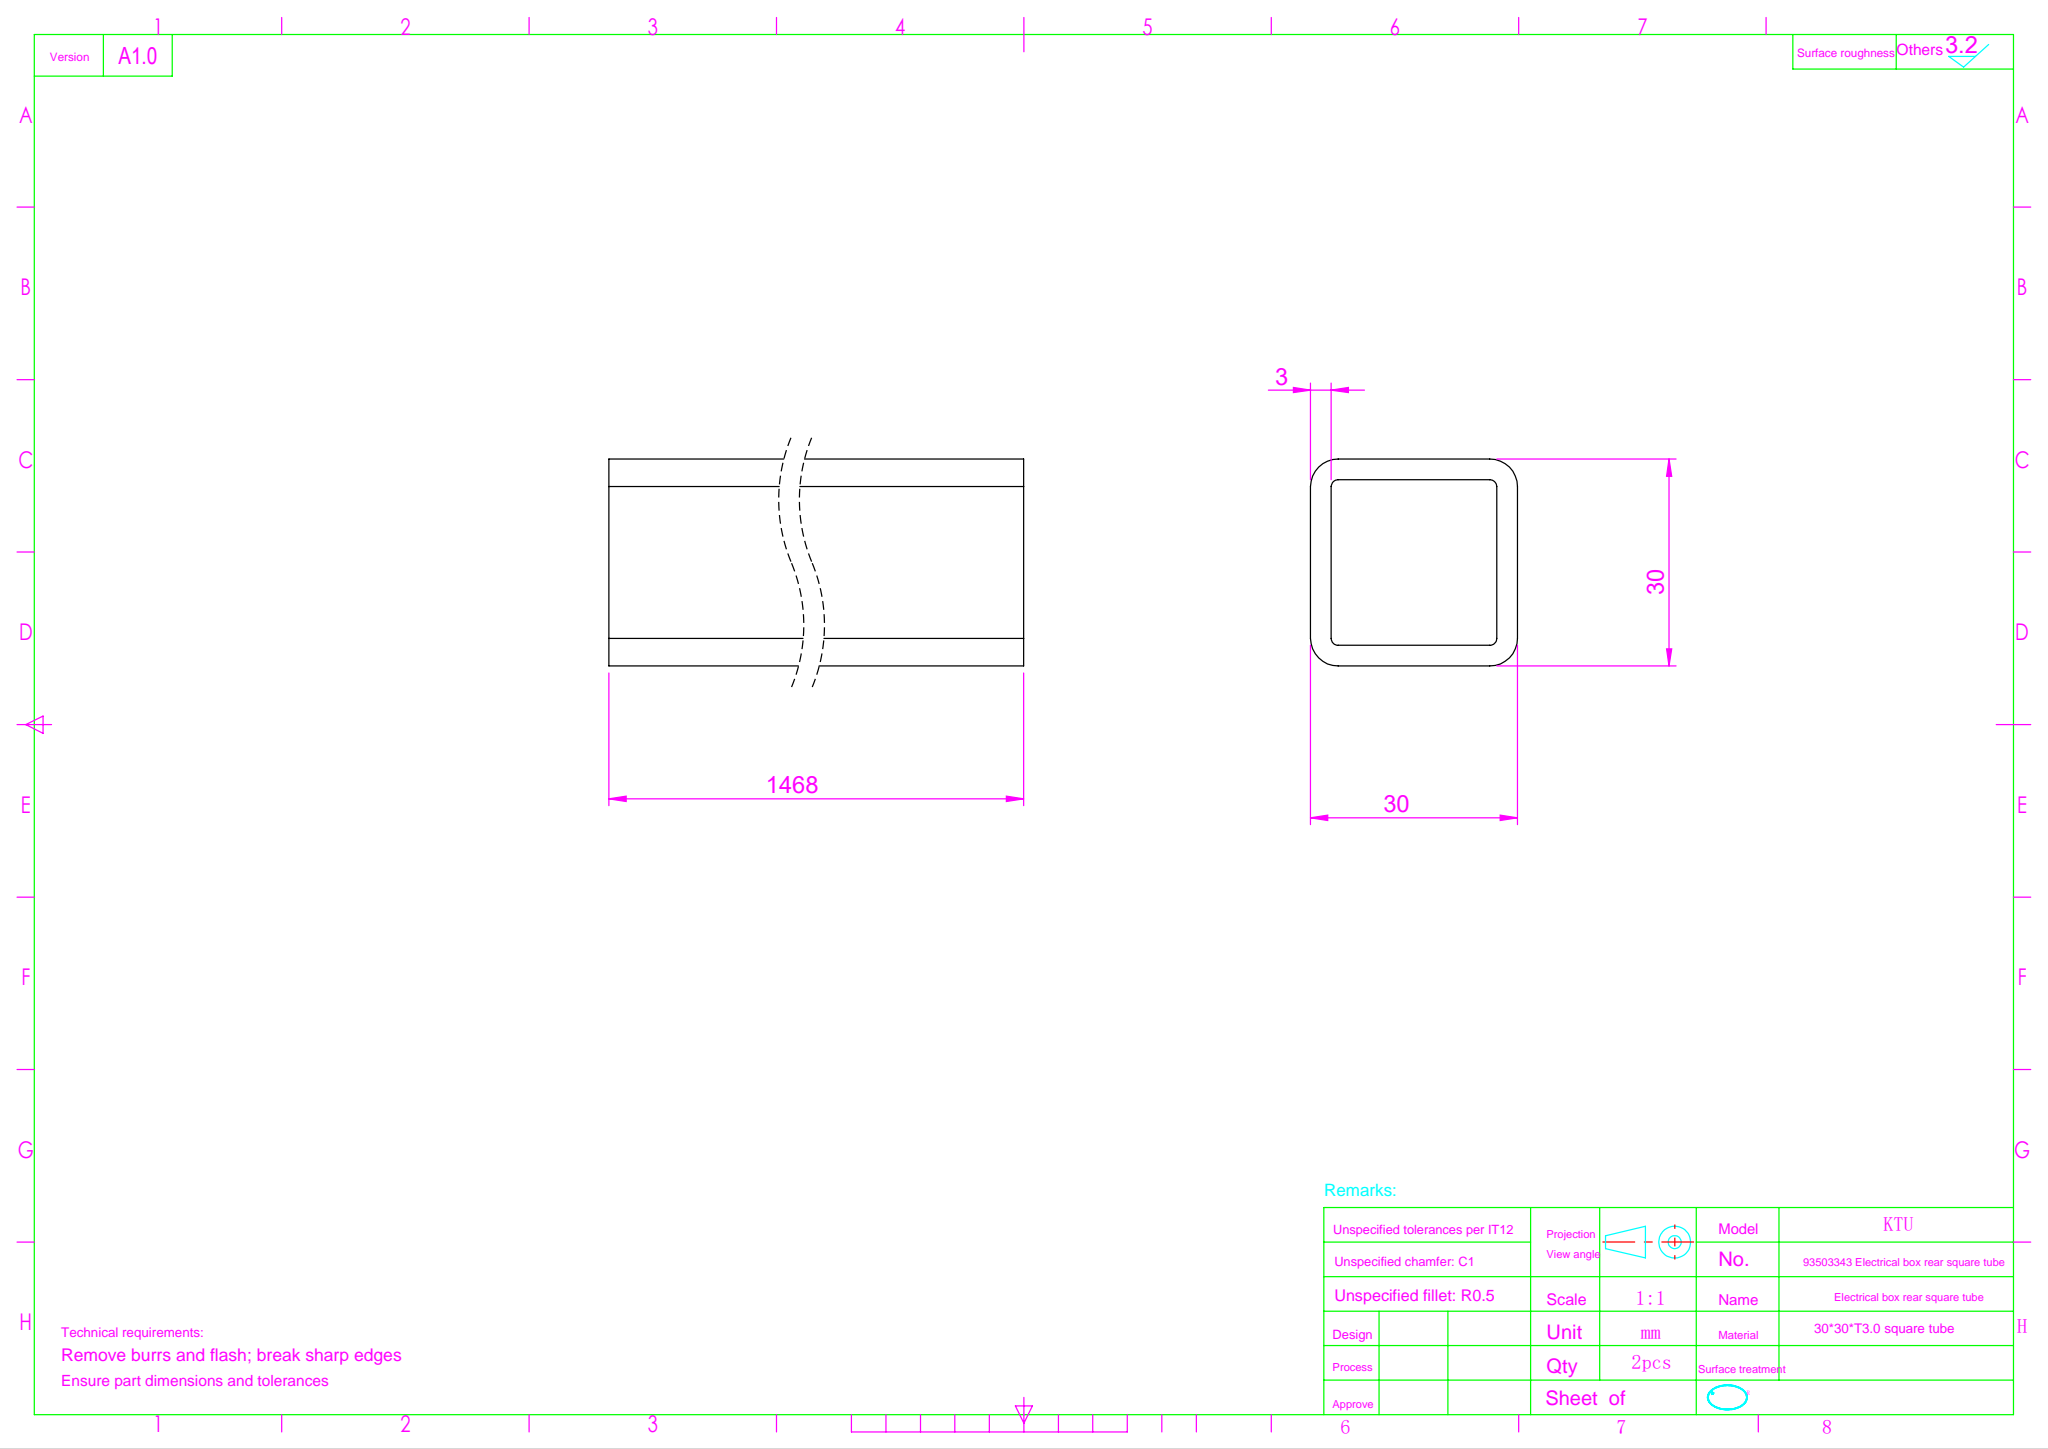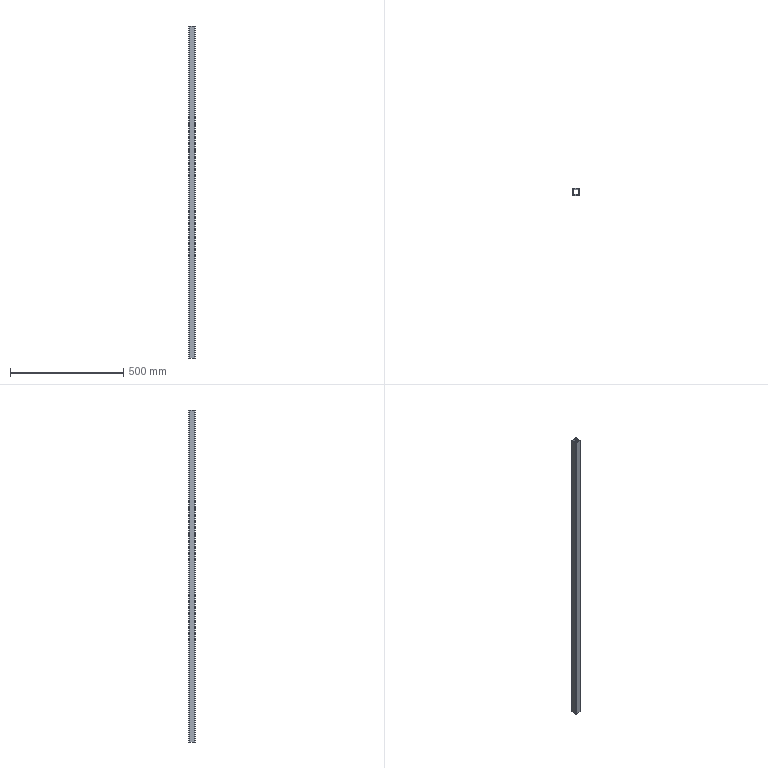Part | SolidWorks | features ExtruThin 1 | 1 solid | 18 faces | box 30 x 30 x 1468 mm | volume 456730 mm3 | plane 10 | cylinder 8 | commonest cylinder face diameters 2 x4 8 x4
STEP:
#1=CARTESIAN_POINT('',(15.,11.,734.));
#2=VERTEX_POINT('',#1);
#3=CARTESIAN_POINT('',(11.,15.,734.));
#4=VERTEX_POINT('',#3);
#5=CARTESIAN_POINT('',(11.,11.,734.));
#6=DIRECTION('',(0.,0.,1.));
#7=DIRECTION('',(-1.,0.,0.));
#8=AXIS2_PLACEMENT_3D('',#5,#6,#7);
#9=CIRCLE('',#8,4.);
#10=EDGE_CURVE('',#2,#4,#9,.T.);
#11=ORIENTED_EDGE('',*,*,#10,.T.);
#12=CARTESIAN_POINT('',(-11.,15.,734.));
#13=VERTEX_POINT('',#12);
#14=CARTESIAN_POINT('',(-11.,15.,734.));
#15=DIRECTION('',(-1.,0.,0.));
#16=VECTOR('',#15,1000.);
#17=LINE('',#14,#16);
#18=EDGE_CURVE('',#4,#13,#17,.T.);
#19=ORIENTED_EDGE('',*,*,#18,.T.);
#20=CARTESIAN_POINT('',(-15.,11.,734.));
#21=VERTEX_POINT('',#20);
#22=CARTESIAN_POINT('',(-11.,11.,734.));
#23=DIRECTION('',(0.,0.,1.));
#24=DIRECTION('',(1.,0.,0.));
#25=AXIS2_PLACEMENT_3D('',#22,#23,#24);
#26=CIRCLE('',#25,4.);
#27=EDGE_CURVE('',#13,#21,#26,.T.);
#28=ORIENTED_EDGE('',*,*,#27,.T.);
#29=CARTESIAN_POINT('',(-15.,-11.,734.));
#30=VERTEX_POINT('',#29);
#31=CARTESIAN_POINT('',(-15.,11.,734.));
#32=DIRECTION('',(0.,-1.,0.));
#33=VECTOR('',#32,1000.);
#34=LINE('',#31,#33);
#35=EDGE_CURVE('',#21,#30,#34,.T.);
#36=ORIENTED_EDGE('',*,*,#35,.T.);
#37=CARTESIAN_POINT('',(-11.,-15.,734.));
#38=VERTEX_POINT('',#37);
#39=CARTESIAN_POINT('',(-11.,-11.,734.));
#40=DIRECTION('',(0.,0.,1.));
#41=DIRECTION('',(1.,0.,0.));
#42=AXIS2_PLACEMENT_3D('',#39,#40,#41);
#43=CIRCLE('',#42,4.);
#44=EDGE_CURVE('',#30,#38,#43,.T.);
#45=ORIENTED_EDGE('',*,*,#44,.T.);
#46=CARTESIAN_POINT('',(11.,-15.,734.));
#47=VERTEX_POINT('',#46);
#48=CARTESIAN_POINT('',(-11.,-15.,734.));
#49=DIRECTION('',(1.,0.,0.));
#50=VECTOR('',#49,1000.);
#51=LINE('',#48,#50);
#52=EDGE_CURVE('',#38,#47,#51,.T.);
#53=ORIENTED_EDGE('',*,*,#52,.T.);
#54=CARTESIAN_POINT('',(15.,-11.,734.));
#55=VERTEX_POINT('',#54);
#56=CARTESIAN_POINT('',(11.,-11.,734.));
#57=DIRECTION('',(0.,0.,1.));
#58=DIRECTION('',(1.,0.,0.));
#59=AXIS2_PLACEMENT_3D('',#56,#57,#58);
#60=CIRCLE('',#59,4.);
#61=EDGE_CURVE('',#47,#55,#60,.T.);
#62=ORIENTED_EDGE('',*,*,#61,.T.);
#63=CARTESIAN_POINT('',(15.,11.,734.));
#64=DIRECTION('',(0.,1.,0.));
#65=VECTOR('',#64,1000.);
#66=LINE('',#63,#65);
#67=EDGE_CURVE('',#55,#2,#66,.T.);
#68=ORIENTED_EDGE('',*,*,#67,.T.);
#69=EDGE_LOOP('',(#11,#19,#28,#36,#45,#53,#62,#68));
#70=FACE_OUTER_BOUND('',#69,.T.);
#71=CARTESIAN_POINT('',(11.,12.,734.));
#72=VERTEX_POINT('',#71);
#73=CARTESIAN_POINT('',(-11.,12.,734.));
#74=VERTEX_POINT('',#73);
#75=CARTESIAN_POINT('',(11.,12.,734.));
#76=DIRECTION('',(-1.,0.,0.));
#77=VECTOR('',#76,1000.);
#78=LINE('',#75,#77);
#79=EDGE_CURVE('',#72,#74,#78,.T.);
#80=ORIENTED_EDGE('',*,*,#79,.F.);
#81=CARTESIAN_POINT('',(12.,11.,734.));
#82=VERTEX_POINT('',#81);
#83=CARTESIAN_POINT('',(11.,11.,734.));
#84=DIRECTION('',(0.,0.,1.));
#85=DIRECTION('',(-1.,0.,0.));
#86=AXIS2_PLACEMENT_3D('',#83,#84,#85);
#87=CIRCLE('',#86,1.);
#88=EDGE_CURVE('',#82,#72,#87,.T.);
#89=ORIENTED_EDGE('',*,*,#88,.F.);
#90=CARTESIAN_POINT('',(12.,-11.,734.));
#91=VERTEX_POINT('',#90);
#92=CARTESIAN_POINT('',(12.,11.,734.));
#93=DIRECTION('',(0.,1.,0.));
#94=VECTOR('',#93,1000.);
#95=LINE('',#92,#94);
#96=EDGE_CURVE('',#91,#82,#95,.T.);
#97=ORIENTED_EDGE('',*,*,#96,.F.);
#98=CARTESIAN_POINT('',(11.,-12.,734.));
#99=VERTEX_POINT('',#98);
#100=CARTESIAN_POINT('',(11.,-11.,734.));
#101=DIRECTION('',(0.,0.,1.));
#102=DIRECTION('',(-1.,0.,0.));
#103=AXIS2_PLACEMENT_3D('',#100,#101,#102);
#104=CIRCLE('',#103,1.);
#105=EDGE_CURVE('',#99,#91,#104,.T.);
#106=ORIENTED_EDGE('',*,*,#105,.F.);
#107=CARTESIAN_POINT('',(-11.,-12.,734.));
#108=VERTEX_POINT('',#107);
#109=CARTESIAN_POINT('',(11.,-12.,734.));
#110=DIRECTION('',(1.,0.,0.));
#111=VECTOR('',#110,1000.);
#112=LINE('',#109,#111);
#113=EDGE_CURVE('',#108,#99,#112,.T.);
#114=ORIENTED_EDGE('',*,*,#113,.F.);
#115=CARTESIAN_POINT('',(-12.,-11.,734.));
#116=VERTEX_POINT('',#115);
#117=CARTESIAN_POINT('',(-11.,-11.,734.));
#118=DIRECTION('',(0.,0.,1.));
#119=DIRECTION('',(-1.,0.,0.));
#120=AXIS2_PLACEMENT_3D('',#117,#118,#119);
#121=CIRCLE('',#120,1.);
#122=EDGE_CURVE('',#116,#108,#121,.T.);
#123=ORIENTED_EDGE('',*,*,#122,.F.);
#124=CARTESIAN_POINT('',(-12.,11.,734.));
#125=VERTEX_POINT('',#124);
#126=CARTESIAN_POINT('',(-12.,11.,734.));
#127=DIRECTION('',(0.,-1.,0.));
#128=VECTOR('',#127,1000.);
#129=LINE('',#126,#128);
#130=EDGE_CURVE('',#125,#116,#129,.T.);
#131=ORIENTED_EDGE('',*,*,#130,.F.);
#132=CARTESIAN_POINT('',(-11.,11.,734.));
#133=DIRECTION('',(0.,0.,1.));
#134=DIRECTION('',(-1.,0.,0.));
#135=AXIS2_PLACEMENT_3D('',#132,#133,#134);
#136=CIRCLE('',#135,1.);
#137=EDGE_CURVE('',#74,#125,#136,.T.);
#138=ORIENTED_EDGE('',*,*,#137,.F.);
#139=EDGE_LOOP('',(#80,#89,#97,#106,#114,#123,#131,#138));
#140=FACE_BOUND('',#139,.T.);
#141=CARTESIAN_POINT('',(11.,11.,734.));
#142=DIRECTION('',(0.,0.,1.));
#143=DIRECTION('',(1.,0.,0.));
#144=AXIS2_PLACEMENT_3D('',#141,#142,#143);
#145=PLANE('',#144);
#146=ADVANCED_FACE('',(#70,#140),#145,.T.);
#147=CARTESIAN_POINT('',(15.,11.,-734.));
#148=VERTEX_POINT('',#147);
#149=CARTESIAN_POINT('',(11.,15.,-734.));
#150=VERTEX_POINT('',#149);
#151=CARTESIAN_POINT('',(11.,11.,-734.));
#152=DIRECTION('',(0.,0.,1.));
#153=DIRECTION('',(-1.,0.,0.));
#154=AXIS2_PLACEMENT_3D('',#151,#152,#153);
#155=CIRCLE('',#154,4.);
#156=EDGE_CURVE('',#148,#150,#155,.T.);
#157=ORIENTED_EDGE('',*,*,#156,.F.);
#158=CARTESIAN_POINT('',(15.,-11.,-734.));
#159=VERTEX_POINT('',#158);
#160=CARTESIAN_POINT('',(15.,11.,-734.));
#161=DIRECTION('',(0.,1.,0.));
#162=VECTOR('',#161,1000.);
#163=LINE('',#160,#162);
#164=EDGE_CURVE('',#159,#148,#163,.T.);
#165=ORIENTED_EDGE('',*,*,#164,.F.);
#166=CARTESIAN_POINT('',(11.,-15.,-734.));
#167=VERTEX_POINT('',#166);
#168=CARTESIAN_POINT('',(11.,-11.,-734.));
#169=DIRECTION('',(0.,0.,1.));
#170=DIRECTION('',(1.,0.,0.));
#171=AXIS2_PLACEMENT_3D('',#168,#169,#170);
#172=CIRCLE('',#171,4.);
#173=EDGE_CURVE('',#167,#159,#172,.T.);
#174=ORIENTED_EDGE('',*,*,#173,.F.);
#175=CARTESIAN_POINT('',(-11.,-15.,-734.));
#176=VERTEX_POINT('',#175);
#177=CARTESIAN_POINT('',(-11.,-15.,-734.));
#178=DIRECTION('',(1.,0.,0.));
#179=VECTOR('',#178,1000.);
#180=LINE('',#177,#179);
#181=EDGE_CURVE('',#176,#167,#180,.T.);
#182=ORIENTED_EDGE('',*,*,#181,.F.);
#183=CARTESIAN_POINT('',(-15.,-11.,-734.));
#184=VERTEX_POINT('',#183);
#185=CARTESIAN_POINT('',(-11.,-11.,-734.));
#186=DIRECTION('',(0.,0.,1.));
#187=DIRECTION('',(1.,0.,0.));
#188=AXIS2_PLACEMENT_3D('',#185,#186,#187);
#189=CIRCLE('',#188,4.);
#190=EDGE_CURVE('',#184,#176,#189,.T.);
#191=ORIENTED_EDGE('',*,*,#190,.F.);
#192=CARTESIAN_POINT('',(-15.,11.,-734.));
#193=VERTEX_POINT('',#192);
#194=CARTESIAN_POINT('',(-15.,11.,-734.));
#195=DIRECTION('',(0.,-1.,0.));
#196=VECTOR('',#195,1000.);
#197=LINE('',#194,#196);
#198=EDGE_CURVE('',#193,#184,#197,.T.);
#199=ORIENTED_EDGE('',*,*,#198,.F.);
#200=CARTESIAN_POINT('',(-11.,15.,-734.));
#201=VERTEX_POINT('',#200);
#202=CARTESIAN_POINT('',(-11.,11.,-734.));
#203=DIRECTION('',(0.,0.,1.));
#204=DIRECTION('',(1.,0.,0.));
#205=AXIS2_PLACEMENT_3D('',#202,#203,#204);
#206=CIRCLE('',#205,4.);
#207=EDGE_CURVE('',#201,#193,#206,.T.);
#208=ORIENTED_EDGE('',*,*,#207,.F.);
#209=CARTESIAN_POINT('',(-11.,15.,-734.));
#210=DIRECTION('',(-1.,0.,0.));
#211=VECTOR('',#210,1000.);
#212=LINE('',#209,#211);
#213=EDGE_CURVE('',#150,#201,#212,.T.);
#214=ORIENTED_EDGE('',*,*,#213,.F.);
#215=EDGE_LOOP('',(#157,#165,#174,#182,#191,#199,#208,#214));
#216=FACE_OUTER_BOUND('',#215,.T.);
#217=CARTESIAN_POINT('',(12.,11.,-734.));
#218=VERTEX_POINT('',#217);
#219=CARTESIAN_POINT('',(11.,12.,-734.));
#220=VERTEX_POINT('',#219);
#221=CARTESIAN_POINT('',(11.,11.,-734.));
#222=DIRECTION('',(0.,0.,1.));
#223=DIRECTION('',(-1.,0.,0.));
#224=AXIS2_PLACEMENT_3D('',#221,#222,#223);
#225=CIRCLE('',#224,1.);
#226=EDGE_CURVE('',#218,#220,#225,.T.);
#227=ORIENTED_EDGE('',*,*,#226,.T.);
#228=CARTESIAN_POINT('',(-11.,12.,-734.));
#229=VERTEX_POINT('',#228);
#230=CARTESIAN_POINT('',(11.,12.,-734.));
#231=DIRECTION('',(-1.,0.,0.));
#232=VECTOR('',#231,1000.);
#233=LINE('',#230,#232);
#234=EDGE_CURVE('',#220,#229,#233,.T.);
#235=ORIENTED_EDGE('',*,*,#234,.T.);
#236=CARTESIAN_POINT('',(-12.,11.,-734.));
#237=VERTEX_POINT('',#236);
#238=CARTESIAN_POINT('',(-11.,11.,-734.));
#239=DIRECTION('',(0.,0.,1.));
#240=DIRECTION('',(-1.,0.,0.));
#241=AXIS2_PLACEMENT_3D('',#238,#239,#240);
#242=CIRCLE('',#241,1.);
#243=EDGE_CURVE('',#229,#237,#242,.T.);
#244=ORIENTED_EDGE('',*,*,#243,.T.);
#245=CARTESIAN_POINT('',(-12.,-11.,-734.));
#246=VERTEX_POINT('',#245);
#247=CARTESIAN_POINT('',(-12.,11.,-734.));
#248=DIRECTION('',(0.,-1.,0.));
#249=VECTOR('',#248,1000.);
#250=LINE('',#247,#249);
#251=EDGE_CURVE('',#237,#246,#250,.T.);
#252=ORIENTED_EDGE('',*,*,#251,.T.);
#253=CARTESIAN_POINT('',(-11.,-12.,-734.));
#254=VERTEX_POINT('',#253);
#255=CARTESIAN_POINT('',(-11.,-11.,-734.));
#256=DIRECTION('',(0.,0.,1.));
#257=DIRECTION('',(-1.,0.,0.));
#258=AXIS2_PLACEMENT_3D('',#255,#256,#257);
#259=CIRCLE('',#258,1.);
#260=EDGE_CURVE('',#246,#254,#259,.T.);
#261=ORIENTED_EDGE('',*,*,#260,.T.);
#262=CARTESIAN_POINT('',(11.,-12.,-734.));
#263=VERTEX_POINT('',#262);
#264=CARTESIAN_POINT('',(11.,-12.,-734.));
#265=DIRECTION('',(1.,0.,0.));
#266=VECTOR('',#265,1000.);
#267=LINE('',#264,#266);
#268=EDGE_CURVE('',#254,#263,#267,.T.);
#269=ORIENTED_EDGE('',*,*,#268,.T.);
#270=CARTESIAN_POINT('',(12.,-11.,-734.));
#271=VERTEX_POINT('',#270);
#272=CARTESIAN_POINT('',(11.,-11.,-734.));
#273=DIRECTION('',(0.,0.,1.));
#274=DIRECTION('',(-1.,0.,0.));
#275=AXIS2_PLACEMENT_3D('',#272,#273,#274);
#276=CIRCLE('',#275,1.);
#277=EDGE_CURVE('',#263,#271,#276,.T.);
#278=ORIENTED_EDGE('',*,*,#277,.T.);
#279=CARTESIAN_POINT('',(12.,11.,-734.));
#280=DIRECTION('',(0.,1.,0.));
#281=VECTOR('',#280,1000.);
#282=LINE('',#279,#281);
#283=EDGE_CURVE('',#271,#218,#282,.T.);
#284=ORIENTED_EDGE('',*,*,#283,.T.);
#285=EDGE_LOOP('',(#227,#235,#244,#252,#261,#269,#278,#284));
#286=FACE_BOUND('',#285,.T.);
#287=CARTESIAN_POINT('',(11.,11.,-734.));
#288=DIRECTION('',(0.,0.,1.));
#289=DIRECTION('',(1.,0.,0.));
#290=AXIS2_PLACEMENT_3D('',#287,#288,#289);
#291=PLANE('',#290);
#292=ADVANCED_FACE('',(#216,#286),#291,.F.);
#293=ORIENTED_EDGE('',*,*,#156,.T.);
#294=CARTESIAN_POINT('',(11.,15.,734.));
#295=DIRECTION('',(0.,0.,-1.));
#296=VECTOR('',#295,1000.);
#297=LINE('',#294,#296);
#298=EDGE_CURVE('',#4,#150,#297,.T.);
#299=ORIENTED_EDGE('',*,*,#298,.F.);
#300=ORIENTED_EDGE('',*,*,#10,.F.);
#301=CARTESIAN_POINT('',(15.,11.,734.));
#302=DIRECTION('',(0.,0.,-1.));
#303=VECTOR('',#302,1000.);
#304=LINE('',#301,#303);
#305=EDGE_CURVE('',#2,#148,#304,.T.);
#306=ORIENTED_EDGE('',*,*,#305,.T.);
#307=EDGE_LOOP('',(#293,#299,#300,#306));
#308=FACE_OUTER_BOUND('',#307,.T.);
#309=CARTESIAN_POINT('',(11.,11.,734.));
#310=DIRECTION('',(0.,0.,-1.));
#311=DIRECTION('',(-1.,0.,0.));
#312=AXIS2_PLACEMENT_3D('',#309,#310,#311);
#313=CYLINDRICAL_SURFACE('',#312,4.);
#314=ADVANCED_FACE('',(#308),#313,.T.);
#315=ORIENTED_EDGE('',*,*,#213,.T.);
#316=CARTESIAN_POINT('',(-11.,15.,734.));
#317=DIRECTION('',(0.,0.,-1.));
#318=VECTOR('',#317,1000.);
#319=LINE('',#316,#318);
#320=EDGE_CURVE('',#13,#201,#319,.T.);
#321=ORIENTED_EDGE('',*,*,#320,.F.);
#322=ORIENTED_EDGE('',*,*,#18,.F.);
#323=ORIENTED_EDGE('',*,*,#298,.T.);
#324=EDGE_LOOP('',(#315,#321,#322,#323));
#325=FACE_OUTER_BOUND('',#324,.T.);
#326=CARTESIAN_POINT('',(-11.,15.,734.));
#327=DIRECTION('',(0.,-1.,0.));
#328=DIRECTION('',(0.,0.,-1.));
#329=AXIS2_PLACEMENT_3D('',#326,#327,#328);
#330=PLANE('',#329);
#331=ADVANCED_FACE('',(#325),#330,.F.);
#332=ORIENTED_EDGE('',*,*,#207,.T.);
#333=CARTESIAN_POINT('',(-15.,11.,734.));
#334=DIRECTION('',(0.,0.,-1.));
#335=VECTOR('',#334,1000.);
#336=LINE('',#333,#335);
#337=EDGE_CURVE('',#21,#193,#336,.T.);
#338=ORIENTED_EDGE('',*,*,#337,.F.);
#339=ORIENTED_EDGE('',*,*,#27,.F.);
#340=ORIENTED_EDGE('',*,*,#320,.T.);
#341=EDGE_LOOP('',(#332,#338,#339,#340));
#342=FACE_OUTER_BOUND('',#341,.T.);
#343=CARTESIAN_POINT('',(-11.,11.,734.));
#344=DIRECTION('',(0.,0.,-1.));
#345=DIRECTION('',(-1.,0.,0.));
#346=AXIS2_PLACEMENT_3D('',#343,#344,#345);
#347=CYLINDRICAL_SURFACE('',#346,4.);
#348=ADVANCED_FACE('',(#342),#347,.T.);
#349=ORIENTED_EDGE('',*,*,#198,.T.);
#350=CARTESIAN_POINT('',(-15.,-11.,734.));
#351=DIRECTION('',(0.,0.,-1.));
#352=VECTOR('',#351,1000.);
#353=LINE('',#350,#352);
#354=EDGE_CURVE('',#30,#184,#353,.T.);
#355=ORIENTED_EDGE('',*,*,#354,.F.);
#356=ORIENTED_EDGE('',*,*,#35,.F.);
#357=ORIENTED_EDGE('',*,*,#337,.T.);
#358=EDGE_LOOP('',(#349,#355,#356,#357));
#359=FACE_OUTER_BOUND('',#358,.T.);
#360=CARTESIAN_POINT('',(-15.,11.,734.));
#361=DIRECTION('',(1.,0.,0.));
#362=DIRECTION('',(0.,1.,0.));
#363=AXIS2_PLACEMENT_3D('',#360,#361,#362);
#364=PLANE('',#363);
#365=ADVANCED_FACE('',(#359),#364,.F.);
#366=ORIENTED_EDGE('',*,*,#190,.T.);
#367=CARTESIAN_POINT('',(-11.,-15.,734.));
#368=DIRECTION('',(0.,0.,-1.));
#369=VECTOR('',#368,1000.);
#370=LINE('',#367,#369);
#371=EDGE_CURVE('',#38,#176,#370,.T.);
#372=ORIENTED_EDGE('',*,*,#371,.F.);
#373=ORIENTED_EDGE('',*,*,#44,.F.);
#374=ORIENTED_EDGE('',*,*,#354,.T.);
#375=EDGE_LOOP('',(#366,#372,#373,#374));
#376=FACE_OUTER_BOUND('',#375,.T.);
#377=CARTESIAN_POINT('',(-11.,-11.,734.));
#378=DIRECTION('',(0.,0.,-1.));
#379=DIRECTION('',(-1.,0.,0.));
#380=AXIS2_PLACEMENT_3D('',#377,#378,#379);
#381=CYLINDRICAL_SURFACE('',#380,4.);
#382=ADVANCED_FACE('',(#376),#381,.T.);
#383=ORIENTED_EDGE('',*,*,#181,.T.);
#384=CARTESIAN_POINT('',(11.,-15.,734.));
#385=DIRECTION('',(0.,0.,-1.));
#386=VECTOR('',#385,1000.);
#387=LINE('',#384,#386);
#388=EDGE_CURVE('',#47,#167,#387,.T.);
#389=ORIENTED_EDGE('',*,*,#388,.F.);
#390=ORIENTED_EDGE('',*,*,#52,.F.);
#391=ORIENTED_EDGE('',*,*,#371,.T.);
#392=EDGE_LOOP('',(#383,#389,#390,#391));
#393=FACE_OUTER_BOUND('',#392,.T.);
#394=CARTESIAN_POINT('',(-11.,-15.,734.));
#395=DIRECTION('',(0.,1.,0.));
#396=DIRECTION('',(0.,0.,1.));
#397=AXIS2_PLACEMENT_3D('',#394,#395,#396);
#398=PLANE('',#397);
#399=ADVANCED_FACE('',(#393),#398,.F.);
#400=ORIENTED_EDGE('',*,*,#173,.T.);
#401=CARTESIAN_POINT('',(15.,-11.,734.));
#402=DIRECTION('',(0.,0.,-1.));
#403=VECTOR('',#402,1000.);
#404=LINE('',#401,#403);
#405=EDGE_CURVE('',#55,#159,#404,.T.);
#406=ORIENTED_EDGE('',*,*,#405,.F.);
#407=ORIENTED_EDGE('',*,*,#61,.F.);
#408=ORIENTED_EDGE('',*,*,#388,.T.);
#409=EDGE_LOOP('',(#400,#406,#407,#408));
#410=FACE_OUTER_BOUND('',#409,.T.);
#411=CARTESIAN_POINT('',(11.,-11.,734.));
#412=DIRECTION('',(0.,0.,-1.));
#413=DIRECTION('',(-1.,0.,0.));
#414=AXIS2_PLACEMENT_3D('',#411,#412,#413);
#415=CYLINDRICAL_SURFACE('',#414,4.);
#416=ADVANCED_FACE('',(#410),#415,.T.);
#417=ORIENTED_EDGE('',*,*,#164,.T.);
#418=ORIENTED_EDGE('',*,*,#305,.F.);
#419=ORIENTED_EDGE('',*,*,#67,.F.);
#420=ORIENTED_EDGE('',*,*,#405,.T.);
#421=EDGE_LOOP('',(#417,#418,#419,#420));
#422=FACE_OUTER_BOUND('',#421,.T.);
#423=CARTESIAN_POINT('',(15.,11.,734.));
#424=DIRECTION('',(-1.,0.,0.));
#425=DIRECTION('',(0.,-1.,0.));
#426=AXIS2_PLACEMENT_3D('',#423,#424,#425);
#427=PLANE('',#426);
#428=ADVANCED_FACE('',(#422),#427,.F.);
#429=ORIENTED_EDGE('',*,*,#226,.F.);
#430=CARTESIAN_POINT('',(12.,11.,734.));
#431=DIRECTION('',(0.,0.,-1.));
#432=VECTOR('',#431,1000.);
#433=LINE('',#430,#432);
#434=EDGE_CURVE('',#82,#218,#433,.T.);
#435=ORIENTED_EDGE('',*,*,#434,.F.);
#436=ORIENTED_EDGE('',*,*,#88,.T.);
#437=CARTESIAN_POINT('',(11.,12.,734.));
#438=DIRECTION('',(0.,0.,-1.));
#439=VECTOR('',#438,1000.);
#440=LINE('',#437,#439);
#441=EDGE_CURVE('',#72,#220,#440,.T.);
#442=ORIENTED_EDGE('',*,*,#441,.T.);
#443=EDGE_LOOP('',(#429,#435,#436,#442));
#444=FACE_OUTER_BOUND('',#443,.T.);
#445=CARTESIAN_POINT('',(11.,11.,734.));
#446=DIRECTION('',(0.,0.,-1.));
#447=DIRECTION('',(-1.,0.,0.));
#448=AXIS2_PLACEMENT_3D('',#445,#446,#447);
#449=CYLINDRICAL_SURFACE('',#448,1.);
#450=ADVANCED_FACE('',(#444),#449,.F.);
#451=ORIENTED_EDGE('',*,*,#234,.F.);
#452=ORIENTED_EDGE('',*,*,#441,.F.);
#453=ORIENTED_EDGE('',*,*,#79,.T.);
#454=CARTESIAN_POINT('',(-11.,12.,734.));
#455=DIRECTION('',(0.,0.,-1.));
#456=VECTOR('',#455,1000.);
#457=LINE('',#454,#456);
#458=EDGE_CURVE('',#74,#229,#457,.T.);
#459=ORIENTED_EDGE('',*,*,#458,.T.);
#460=EDGE_LOOP('',(#451,#452,#453,#459));
#461=FACE_OUTER_BOUND('',#460,.T.);
#462=CARTESIAN_POINT('',(11.,12.,734.));
#463=DIRECTION('',(0.,-1.,0.));
#464=DIRECTION('',(0.,0.,-1.));
#465=AXIS2_PLACEMENT_3D('',#462,#463,#464);
#466=PLANE('',#465);
#467=ADVANCED_FACE('',(#461),#466,.T.);
#468=ORIENTED_EDGE('',*,*,#243,.F.);
#469=ORIENTED_EDGE('',*,*,#458,.F.);
#470=ORIENTED_EDGE('',*,*,#137,.T.);
#471=CARTESIAN_POINT('',(-12.,11.,734.));
#472=DIRECTION('',(0.,0.,-1.));
#473=VECTOR('',#472,1000.);
#474=LINE('',#471,#473);
#475=EDGE_CURVE('',#125,#237,#474,.T.);
#476=ORIENTED_EDGE('',*,*,#475,.T.);
#477=EDGE_LOOP('',(#468,#469,#470,#476));
#478=FACE_OUTER_BOUND('',#477,.T.);
#479=CARTESIAN_POINT('',(-11.,11.,734.));
#480=DIRECTION('',(0.,0.,-1.));
#481=DIRECTION('',(-1.,0.,0.));
#482=AXIS2_PLACEMENT_3D('',#479,#480,#481);
#483=CYLINDRICAL_SURFACE('',#482,1.);
#484=ADVANCED_FACE('',(#478),#483,.F.);
#485=ORIENTED_EDGE('',*,*,#251,.F.);
#486=ORIENTED_EDGE('',*,*,#475,.F.);
#487=ORIENTED_EDGE('',*,*,#130,.T.);
#488=CARTESIAN_POINT('',(-12.,-11.,734.));
#489=DIRECTION('',(0.,0.,-1.));
#490=VECTOR('',#489,1000.);
#491=LINE('',#488,#490);
#492=EDGE_CURVE('',#116,#246,#491,.T.);
#493=ORIENTED_EDGE('',*,*,#492,.T.);
#494=EDGE_LOOP('',(#485,#486,#487,#493));
#495=FACE_OUTER_BOUND('',#494,.T.);
#496=CARTESIAN_POINT('',(-12.,11.,734.));
#497=DIRECTION('',(1.,0.,0.));
#498=DIRECTION('',(0.,1.,0.));
#499=AXIS2_PLACEMENT_3D('',#496,#497,#498);
#500=PLANE('',#499);
#501=ADVANCED_FACE('',(#495),#500,.T.);
#502=ORIENTED_EDGE('',*,*,#260,.F.);
#503=ORIENTED_EDGE('',*,*,#492,.F.);
#504=ORIENTED_EDGE('',*,*,#122,.T.);
#505=CARTESIAN_POINT('',(-11.,-12.,734.));
#506=DIRECTION('',(0.,0.,-1.));
#507=VECTOR('',#506,1000.);
#508=LINE('',#505,#507);
#509=EDGE_CURVE('',#108,#254,#508,.T.);
#510=ORIENTED_EDGE('',*,*,#509,.T.);
#511=EDGE_LOOP('',(#502,#503,#504,#510));
#512=FACE_OUTER_BOUND('',#511,.T.);
#513=CARTESIAN_POINT('',(-11.,-11.,734.));
#514=DIRECTION('',(0.,0.,-1.));
#515=DIRECTION('',(-1.,0.,0.));
#516=AXIS2_PLACEMENT_3D('',#513,#514,#515);
#517=CYLINDRICAL_SURFACE('',#516,1.);
#518=ADVANCED_FACE('',(#512),#517,.F.);
#519=ORIENTED_EDGE('',*,*,#268,.F.);
#520=ORIENTED_EDGE('',*,*,#509,.F.);
#521=ORIENTED_EDGE('',*,*,#113,.T.);
#522=CARTESIAN_POINT('',(11.,-12.,734.));
#523=DIRECTION('',(0.,0.,-1.));
#524=VECTOR('',#523,1000.);
#525=LINE('',#522,#524);
#526=EDGE_CURVE('',#99,#263,#525,.T.);
#527=ORIENTED_EDGE('',*,*,#526,.T.);
#528=EDGE_LOOP('',(#519,#520,#521,#527));
#529=FACE_OUTER_BOUND('',#528,.T.);
#530=CARTESIAN_POINT('',(11.,-12.,734.));
#531=DIRECTION('',(0.,1.,0.));
#532=DIRECTION('',(0.,0.,1.));
#533=AXIS2_PLACEMENT_3D('',#530,#531,#532);
#534=PLANE('',#533);
#535=ADVANCED_FACE('',(#529),#534,.T.);
#536=ORIENTED_EDGE('',*,*,#277,.F.);
#537=ORIENTED_EDGE('',*,*,#526,.F.);
#538=ORIENTED_EDGE('',*,*,#105,.T.);
#539=CARTESIAN_POINT('',(12.,-11.,734.));
#540=DIRECTION('',(0.,0.,-1.));
#541=VECTOR('',#540,1000.);
#542=LINE('',#539,#541);
#543=EDGE_CURVE('',#91,#271,#542,.T.);
#544=ORIENTED_EDGE('',*,*,#543,.T.);
#545=EDGE_LOOP('',(#536,#537,#538,#544));
#546=FACE_OUTER_BOUND('',#545,.T.);
#547=CARTESIAN_POINT('',(11.,-11.,734.));
#548=DIRECTION('',(0.,0.,-1.));
#549=DIRECTION('',(-1.,0.,0.));
#550=AXIS2_PLACEMENT_3D('',#547,#548,#549);
#551=CYLINDRICAL_SURFACE('',#550,1.);
#552=ADVANCED_FACE('',(#546),#551,.F.);
#553=ORIENTED_EDGE('',*,*,#283,.F.);
#554=ORIENTED_EDGE('',*,*,#543,.F.);
#555=ORIENTED_EDGE('',*,*,#96,.T.);
#556=ORIENTED_EDGE('',*,*,#434,.T.);
#557=EDGE_LOOP('',(#553,#554,#555,#556));
#558=FACE_OUTER_BOUND('',#557,.T.);
#559=CARTESIAN_POINT('',(12.,11.,734.));
#560=DIRECTION('',(-1.,0.,0.));
#561=DIRECTION('',(0.,-1.,0.));
#562=AXIS2_PLACEMENT_3D('',#559,#560,#561);
#563=PLANE('',#562);
#564=ADVANCED_FACE('',(#558),#563,.T.);
#565=CLOSED_SHELL('',(#146,#292,#314,#331,#348,#365,#382,#399,#416,#428,#450,#467,#484,#501,#518,#535,#552,#564));
#566=MANIFOLD_SOLID_BREP('',#565);
#567=CARTESIAN_POINT('',(0.,0.,0.));
#568=DIRECTION('',(0.,0.,1.));
#569=DIRECTION('',(1.,0.,0.));
#570=AXIS2_PLACEMENT_3D('',#567,#568,#569);
#571=(LENGTH_UNIT()NAMED_UNIT(*)SI_UNIT(.MILLI.,.METRE.));
#572=UNCERTAINTY_MEASURE_WITH_UNIT(LENGTH_MEASURE(0.00001),#571,'','');
#573=(NAMED_UNIT(*)PLANE_ANGLE_UNIT()SI_UNIT($,.RADIAN.));
#574=(NAMED_UNIT(*)SI_UNIT($,.STERADIAN.)SOLID_ANGLE_UNIT());
#575=(GEOMETRIC_REPRESENTATION_CONTEXT(3)GLOBAL_UNCERTAINTY_ASSIGNED_CONTEXT((#572))GLOBAL_UNIT_ASSIGNED_CONTEXT((#571,#573,#574))REPRESENTATION_CONTEXT('',''));
#576=ADVANCED_BREP_SHAPE_REPRESENTATION('',(#566,#570),#575);